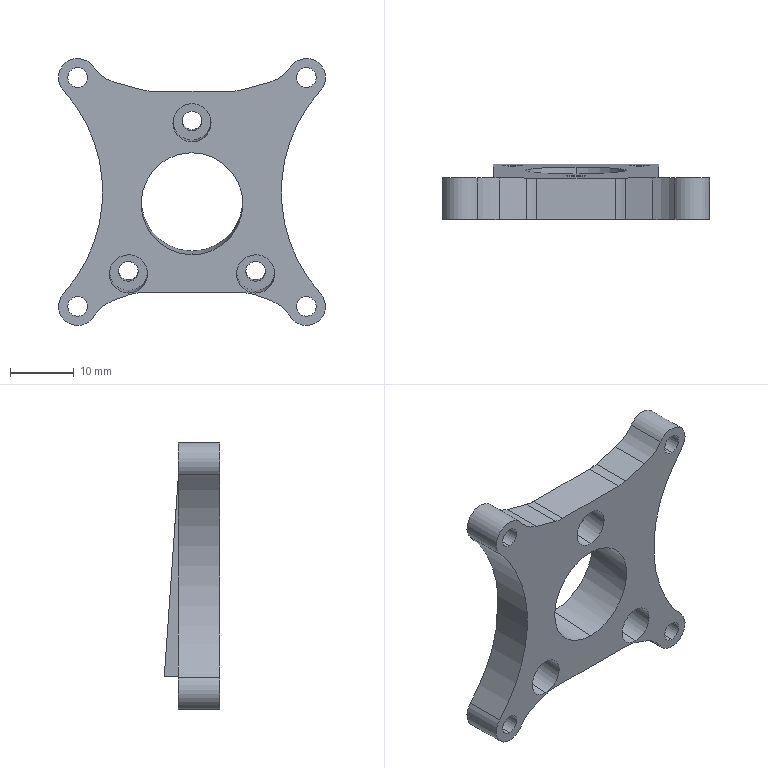Part | SolidWorks | features ICE 3, Extrusion 1, Fillet 1 | 1 solid | 53 faces | box 42 x 8.717 x 42 mm | volume 6163 mm3 | cylinder 38 | plane 15 | commonest cylinder face diameters 3.1 x14 6 x12 12 x8 16 x2 47.629 x2